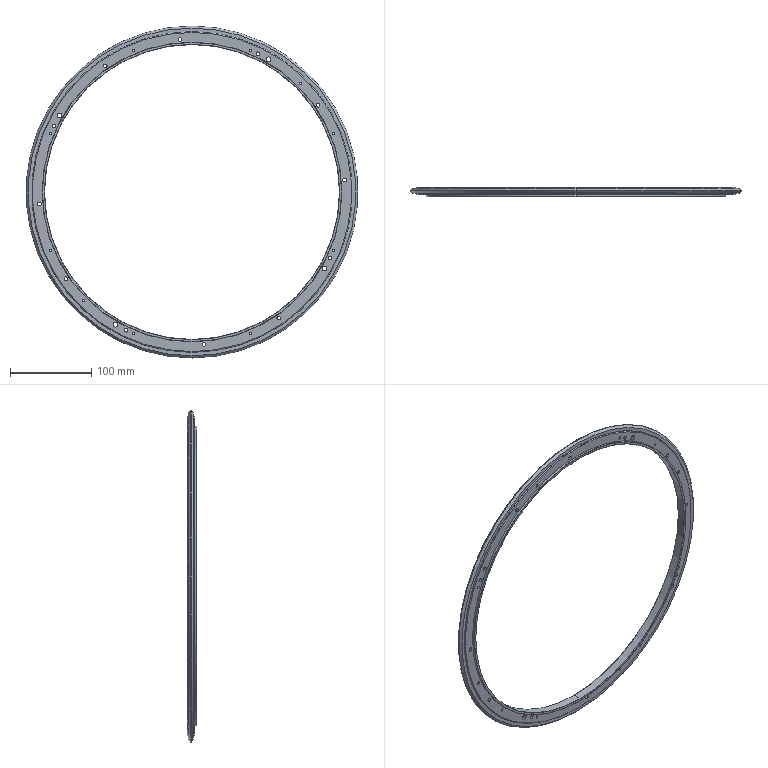Part | NX | features BREP 1 | 1 solid | 137 faces | box 408.8 x 11.6 x 408.8 mm | volume 208158 mm3 | cylinder 98 | plane 21 | cone 18 | commonest cylinder face diameters 4.5 x24 8 x24 3.3 x16 3 x8 6 x8 11 x8